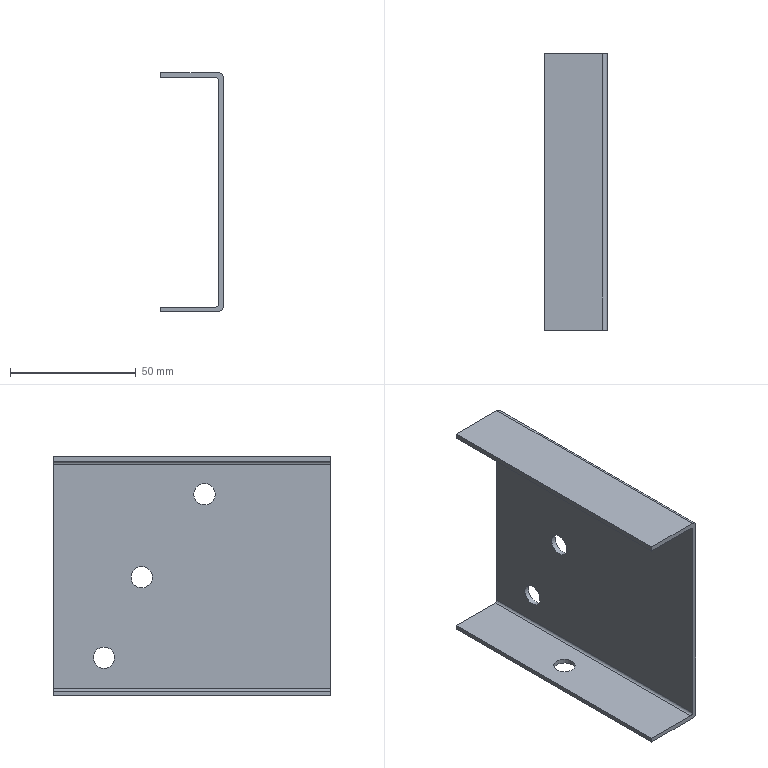Part | STEP file | PN_0066 | 1 solid | 18 faces | box 25 x 110 x 95 mm | volume 29808 mm3 | plane 10 | cylinder 8 | commonest cylinder face diameters 8.5 x4 2 x2 4 x2
STEP:
#1=CARTESIAN_POINT('',(0.,0.,0.));
#2=DIRECTION('',(0.,0.,1.));
#3=DIRECTION('',(1.,0.,0.));
#4=AXIS2_PLACEMENT_3D('',#1,#2,#3);
#5=CARTESIAN_POINT('',(-41.283,0.,45.169));
#6=VERTEX_POINT('',#5);
#7=CARTESIAN_POINT('',(-41.283,0.,43.169));
#8=VERTEX_POINT('',#7);
#9=CARTESIAN_POINT('',(-41.283,0.,43.169));
#10=DIRECTION('',(0.,0.,-1.));
#11=VECTOR('',#10,1.);
#12=LINE('',#9,#11);
#13=CARTESIAN_POINT('',(-41.283,110.,43.169));
#14=DIRECTION('',(1.,0.,0.));
#15=DIRECTION('',(0.,0.,1.));
#16=AXIS2_PLACEMENT_3D('',#13,#14,#15);
#17=PLANE('',#16);
#18=CARTESIAN_POINT('',(0.,110.));
#19=DIRECTION('',(-1.,0.));
#20=VECTOR('',#19,1.);
#21=LINE('',#18,#20);
#22=(GEOMETRIC_REPRESENTATION_CONTEXT(2)PARAMETRIC_REPRESENTATION_CONTEXT()REPRESENTATION_CONTEXT('',''));
#23=DEFINITIONAL_REPRESENTATION('',(#21),#22);
#24=PCURVE('',#17,#23);
#25=CARTESIAN_POINT('',(-18.283,0.,43.169));
#26=DIRECTION('',(0.,1.,0.));
#27=DIRECTION('',(0.,0.,1.));
#28=AXIS2_PLACEMENT_3D('',#25,#26,#27);
#29=PLANE('',#28);
#30=CARTESIAN_POINT('',(0.,-23.));
#31=DIRECTION('',(-1.,0.));
#32=VECTOR('',#31,1.);
#33=LINE('',#30,#32);
#34=(GEOMETRIC_REPRESENTATION_CONTEXT(2)PARAMETRIC_REPRESENTATION_CONTEXT()REPRESENTATION_CONTEXT('',''));
#35=DEFINITIONAL_REPRESENTATION('',(#33),#34);
#36=PCURVE('',#29,#35);
#37=SURFACE_CURVE('',#12,(#24,#36),.PCURVE_S1.);
#38=EDGE_CURVE('',#6,#8,#37,.T.);
#39=ORIENTED_EDGE('',*,*,#38,.F.);
#40=CARTESIAN_POINT('',(-41.283,110.,45.169));
#41=VERTEX_POINT('',#40);
#42=CARTESIAN_POINT('',(-41.283,110.,45.169));
#43=DIRECTION('',(0.,-1.,0.));
#44=VECTOR('',#43,1.);
#45=LINE('',#42,#44);
#46=CARTESIAN_POINT('',(2.,0.));
#47=DIRECTION('',(0.,1.));
#48=VECTOR('',#47,1.);
#49=LINE('',#46,#48);
#50=(GEOMETRIC_REPRESENTATION_CONTEXT(2)PARAMETRIC_REPRESENTATION_CONTEXT()REPRESENTATION_CONTEXT('',''));
#51=DEFINITIONAL_REPRESENTATION('',(#49),#50);
#52=PCURVE('',#17,#51);
#53=CARTESIAN_POINT('',(-18.283,110.,45.169));
#54=DIRECTION('',(0.,0.,-1.));
#55=DIRECTION('',(1.,0.,0.));
#56=AXIS2_PLACEMENT_3D('',#53,#54,#55);
#57=PLANE('',#56);
#58=CARTESIAN_POINT('',(-23.,0.));
#59=DIRECTION('',(0.,1.));
#60=VECTOR('',#59,1.);
#61=LINE('',#58,#60);
#62=(GEOMETRIC_REPRESENTATION_CONTEXT(2)PARAMETRIC_REPRESENTATION_CONTEXT()REPRESENTATION_CONTEXT('',''));
#63=DEFINITIONAL_REPRESENTATION('',(#61),#62);
#64=PCURVE('',#57,#63);
#65=SURFACE_CURVE('',#45,(#52,#64),.PCURVE_S1.);
#66=EDGE_CURVE('',#41,#6,#65,.T.);
#67=ORIENTED_EDGE('',*,*,#66,.F.);
#68=CARTESIAN_POINT('',(-41.283,110.,43.169));
#69=VERTEX_POINT('',#68);
#70=CARTESIAN_POINT('',(-41.283,110.,43.169));
#71=DIRECTION('',(0.,0.,-1.));
#72=VECTOR('',#71,1.);
#73=LINE('',#70,#72);
#74=CARTESIAN_POINT('',(0.,0.));
#75=DIRECTION('',(-1.,0.));
#76=VECTOR('',#75,1.);
#77=LINE('',#74,#76);
#78=(GEOMETRIC_REPRESENTATION_CONTEXT(2)PARAMETRIC_REPRESENTATION_CONTEXT()REPRESENTATION_CONTEXT('',''));
#79=DEFINITIONAL_REPRESENTATION('',(#77),#78);
#80=PCURVE('',#17,#79);
#81=CARTESIAN_POINT('',(-18.283,110.,43.169));
#82=DIRECTION('',(0.,1.,0.));
#83=DIRECTION('',(0.,0.,1.));
#84=AXIS2_PLACEMENT_3D('',#81,#82,#83);
#85=PLANE('',#84);
#86=CARTESIAN_POINT('',(0.,-23.));
#87=DIRECTION('',(-1.,0.));
#88=VECTOR('',#87,1.);
#89=LINE('',#86,#88);
#90=(GEOMETRIC_REPRESENTATION_CONTEXT(2)PARAMETRIC_REPRESENTATION_CONTEXT()REPRESENTATION_CONTEXT('',''));
#91=DEFINITIONAL_REPRESENTATION('',(#89),#90);
#92=PCURVE('',#85,#91);
#93=SURFACE_CURVE('',#73,(#80,#92),.PCURVE_S1.);
#94=EDGE_CURVE('',#41,#69,#93,.T.);
#95=ORIENTED_EDGE('',*,*,#94,.T.);
#96=CARTESIAN_POINT('',(-41.283,110.,43.169));
#97=DIRECTION('',(0.,-1.,0.));
#98=VECTOR('',#97,1.);
#99=LINE('',#96,#98);
#100=CARTESIAN_POINT('',(0.,0.));
#101=DIRECTION('',(0.,1.));
#102=VECTOR('',#101,1.);
#103=LINE('',#100,#102);
#104=(GEOMETRIC_REPRESENTATION_CONTEXT(2)PARAMETRIC_REPRESENTATION_CONTEXT()REPRESENTATION_CONTEXT('',''));
#105=DEFINITIONAL_REPRESENTATION('',(#103),#104);
#106=PCURVE('',#17,#105);
#107=CARTESIAN_POINT('',(-19.283,110.,43.169));
#108=DIRECTION('',(0.,0.,1.));
#109=DIRECTION('',(-1.,0.,0.));
#110=AXIS2_PLACEMENT_3D('',#107,#108,#109);
#111=PLANE('',#110);
#112=CARTESIAN_POINT('',(22.,0.));
#113=DIRECTION('',(0.,1.));
#114=VECTOR('',#113,1.);
#115=LINE('',#112,#114);
#116=(GEOMETRIC_REPRESENTATION_CONTEXT(2)PARAMETRIC_REPRESENTATION_CONTEXT()REPRESENTATION_CONTEXT('',''));
#117=DEFINITIONAL_REPRESENTATION('',(#115),#116);
#118=PCURVE('',#111,#117);
#119=SURFACE_CURVE('',#99,(#106,#118),.PCURVE_S1.);
#120=EDGE_CURVE('',#69,#8,#119,.T.);
#121=ORIENTED_EDGE('',*,*,#120,.T.);
#122=EDGE_LOOP('',(#39,#67,#95,#121));
#123=FACE_BOUND('',#122,.T.);
#124=ADVANCED_FACE('',(#123),#17,.F.);
#125=CARTESIAN_POINT('',(-19.283,0.,43.169));
#126=VERTEX_POINT('',#125);
#127=CARTESIAN_POINT('',(-19.283,0.,43.169));
#128=DIRECTION('',(1.,0.,0.));
#129=VECTOR('',#128,1.);
#130=LINE('',#127,#129);
#131=CARTESIAN_POINT('',(0.,110.));
#132=DIRECTION('',(-1.,0.));
#133=VECTOR('',#132,1.);
#134=LINE('',#131,#133);
#135=(GEOMETRIC_REPRESENTATION_CONTEXT(2)PARAMETRIC_REPRESENTATION_CONTEXT()REPRESENTATION_CONTEXT('',''));
#136=DEFINITIONAL_REPRESENTATION('',(#134),#135);
#137=PCURVE('',#111,#136);
#138=CARTESIAN_POINT('',(0.,-1.));
#139=DIRECTION('',(0.,1.));
#140=VECTOR('',#139,1.);
#141=LINE('',#138,#140);
#142=(GEOMETRIC_REPRESENTATION_CONTEXT(2)PARAMETRIC_REPRESENTATION_CONTEXT()REPRESENTATION_CONTEXT('',''));
#143=DEFINITIONAL_REPRESENTATION('',(#141),#142);
#144=PCURVE('',#29,#143);
#145=SURFACE_CURVE('',#130,(#137,#144),.PCURVE_S1.);
#146=EDGE_CURVE('',#8,#126,#145,.T.);
#147=ORIENTED_EDGE('',*,*,#146,.F.);
#148=ORIENTED_EDGE('',*,*,#120,.F.);
#149=CARTESIAN_POINT('',(-19.283,110.,43.169));
#150=VERTEX_POINT('',#149);
#151=CARTESIAN_POINT('',(-19.283,110.,43.169));
#152=DIRECTION('',(1.,0.,0.));
#153=VECTOR('',#152,1.);
#154=LINE('',#151,#153);
#155=CARTESIAN_POINT('',(0.,0.));
#156=DIRECTION('',(-1.,0.));
#157=VECTOR('',#156,1.);
#158=LINE('',#155,#157);
#159=(GEOMETRIC_REPRESENTATION_CONTEXT(2)PARAMETRIC_REPRESENTATION_CONTEXT()REPRESENTATION_CONTEXT('',''));
#160=DEFINITIONAL_REPRESENTATION('',(#158),#159);
#161=PCURVE('',#111,#160);
#162=CARTESIAN_POINT('',(0.,-1.));
#163=DIRECTION('',(0.,1.));
#164=VECTOR('',#163,1.);
#165=LINE('',#162,#164);
#166=(GEOMETRIC_REPRESENTATION_CONTEXT(2)PARAMETRIC_REPRESENTATION_CONTEXT()REPRESENTATION_CONTEXT('',''));
#167=DEFINITIONAL_REPRESENTATION('',(#165),#166);
#168=PCURVE('',#85,#167);
#169=SURFACE_CURVE('',#154,(#161,#168),.PCURVE_S1.);
#170=EDGE_CURVE('',#69,#150,#169,.T.);
#171=ORIENTED_EDGE('',*,*,#170,.T.);
#172=CARTESIAN_POINT('',(-19.283,110.,43.169));
#173=DIRECTION('',(0.,-1.,0.));
#174=VECTOR('',#173,1.);
#175=LINE('',#172,#174);
#176=CARTESIAN_POINT('',(0.,0.));
#177=DIRECTION('',(0.,1.));
#178=VECTOR('',#177,1.);
#179=LINE('',#176,#178);
#180=(GEOMETRIC_REPRESENTATION_CONTEXT(2)PARAMETRIC_REPRESENTATION_CONTEXT()REPRESENTATION_CONTEXT('',''));
#181=DEFINITIONAL_REPRESENTATION('',(#179),#180);
#182=PCURVE('',#111,#181);
#183=CARTESIAN_POINT('',(-19.283,110.,42.169));
#184=DIRECTION('',(0.,-1.,0.));
#185=DIRECTION('',(0.,0.,-1.));
#186=AXIS2_PLACEMENT_3D('',#183,#184,#185);
#187=CYLINDRICAL_SURFACE('',#186,1.);
#188=CARTESIAN_POINT('',(3.142,0.));
#189=DIRECTION('',(0.,1.));
#190=VECTOR('',#189,1.);
#191=LINE('',#188,#190);
#192=(GEOMETRIC_REPRESENTATION_CONTEXT(2)PARAMETRIC_REPRESENTATION_CONTEXT()REPRESENTATION_CONTEXT('',''));
#193=DEFINITIONAL_REPRESENTATION('',(#191),#192);
#194=PCURVE('',#187,#193);
#195=SURFACE_CURVE('',#175,(#182,#194),.PCURVE_S1.);
#196=EDGE_CURVE('',#150,#126,#195,.T.);
#197=ORIENTED_EDGE('',*,*,#196,.T.);
#198=EDGE_LOOP('',(#147,#148,#171,#197));
#199=FACE_BOUND('',#198,.T.);
#200=ADVANCED_FACE('',(#199),#111,.F.);
#201=CARTESIAN_POINT('',(-18.283,110.,42.169));
#202=VERTEX_POINT('',#201);
#203=CARTESIAN_POINT('',(-18.283,0.,42.169));
#204=VERTEX_POINT('',#203);
#205=CARTESIAN_POINT('',(-18.283,110.,42.169));
#206=DIRECTION('',(0.,-1.,0.));
#207=VECTOR('',#206,1.);
#208=LINE('',#205,#207);
#209=CARTESIAN_POINT('',(1.571,0.));
#210=DIRECTION('',(0.,1.));
#211=VECTOR('',#210,1.);
#212=LINE('',#209,#211);
#213=(GEOMETRIC_REPRESENTATION_CONTEXT(2)PARAMETRIC_REPRESENTATION_CONTEXT()REPRESENTATION_CONTEXT('',''));
#214=DEFINITIONAL_REPRESENTATION('',(#212),#213);
#215=PCURVE('',#187,#214);
#216=CARTESIAN_POINT('',(-18.283,110.,-47.08));
#217=DIRECTION('',(1.,0.,0.));
#218=DIRECTION('',(0.,0.,1.));
#219=AXIS2_PLACEMENT_3D('',#216,#217,#218);
#220=PLANE('',#219);
#221=CARTESIAN_POINT('',(89.249,0.));
#222=DIRECTION('',(0.,1.));
#223=VECTOR('',#222,1.);
#224=LINE('',#221,#223);
#225=(GEOMETRIC_REPRESENTATION_CONTEXT(2)PARAMETRIC_REPRESENTATION_CONTEXT()REPRESENTATION_CONTEXT('',''));
#226=DEFINITIONAL_REPRESENTATION('',(#224),#225);
#227=PCURVE('',#220,#226);
#228=SURFACE_CURVE('',#208,(#215,#227),.PCURVE_S1.);
#229=EDGE_CURVE('',#202,#204,#228,.T.);
#230=ORIENTED_EDGE('',*,*,#229,.F.);
#231=CARTESIAN_POINT('',(-19.283,110.,42.169));
#232=DIRECTION('',(0.,1.,0.));
#233=DIRECTION('',(0.,0.,1.));
#234=AXIS2_PLACEMENT_3D('',#231,#232,#233);
#235=CIRCLE('',#234,1.);
#236=CARTESIAN_POINT('',(3.142,0.));
#237=DIRECTION('',(-1.,0.));
#238=VECTOR('',#237,1.);
#239=LINE('',#236,#238);
#240=(GEOMETRIC_REPRESENTATION_CONTEXT(2)PARAMETRIC_REPRESENTATION_CONTEXT()REPRESENTATION_CONTEXT('',''));
#241=DEFINITIONAL_REPRESENTATION('',(#239),#240);
#242=PCURVE('',#187,#241);
#243=CARTESIAN_POINT('',(-1.,-1.));
#244=DIRECTION('',(1.,0.));
#245=AXIS2_PLACEMENT_2D('',#243,#244);
#246=CIRCLE('',#245,1.);
#247=(GEOMETRIC_REPRESENTATION_CONTEXT(2)PARAMETRIC_REPRESENTATION_CONTEXT()REPRESENTATION_CONTEXT('',''));
#248=DEFINITIONAL_REPRESENTATION('',(#246),#247);
#249=PCURVE('',#85,#248);
#250=SURFACE_CURVE('',#235,(#242,#249),.PCURVE_S1.);
#251=EDGE_CURVE('',#150,#202,#250,.T.);
#252=ORIENTED_EDGE('',*,*,#251,.F.);
#253=ORIENTED_EDGE('',*,*,#196,.T.);
#254=CARTESIAN_POINT('',(-19.283,0.,42.169));
#255=DIRECTION('',(0.,1.,0.));
#256=DIRECTION('',(0.,0.,1.));
#257=AXIS2_PLACEMENT_3D('',#254,#255,#256);
#258=CIRCLE('',#257,1.);
#259=CARTESIAN_POINT('',(3.142,110.));
#260=DIRECTION('',(-1.,0.));
#261=VECTOR('',#260,1.);
#262=LINE('',#259,#261);
#263=(GEOMETRIC_REPRESENTATION_CONTEXT(2)PARAMETRIC_REPRESENTATION_CONTEXT()REPRESENTATION_CONTEXT('',''));
#264=DEFINITIONAL_REPRESENTATION('',(#262),#263);
#265=PCURVE('',#187,#264);
#266=CARTESIAN_POINT('',(-1.,-1.));
#267=DIRECTION('',(1.,0.));
#268=AXIS2_PLACEMENT_2D('',#266,#267);
#269=CIRCLE('',#268,1.);
#270=(GEOMETRIC_REPRESENTATION_CONTEXT(2)PARAMETRIC_REPRESENTATION_CONTEXT()REPRESENTATION_CONTEXT('',''));
#271=DEFINITIONAL_REPRESENTATION('',(#269),#270);
#272=PCURVE('',#29,#271);
#273=SURFACE_CURVE('',#258,(#265,#272),.PCURVE_S1.);
#274=EDGE_CURVE('',#126,#204,#273,.T.);
#275=ORIENTED_EDGE('',*,*,#274,.T.);
#276=EDGE_LOOP('',(#230,#252,#253,#275));
#277=FACE_BOUND('',#276,.F.);
#278=ADVANCED_FACE('',(#277),#187,.F.);
#279=CARTESIAN_POINT('',(-18.283,75.,-7.081));
#280=VERTEX_POINT('',#279);
#281=CARTESIAN_POINT('',(-18.283,75.,-2.831));
#282=DIRECTION('',(1.,0.,0.));
#283=DIRECTION('',(0.,0.,-1.));
#284=AXIS2_PLACEMENT_3D('',#281,#282,#283);
#285=CIRCLE('',#284,4.25);
#286=CARTESIAN_POINT('',(44.249,35.));
#287=DIRECTION('',(-1.,0.));
#288=AXIS2_PLACEMENT_2D('',#286,#287);
#289=CIRCLE('',#288,4.25);
#290=(GEOMETRIC_REPRESENTATION_CONTEXT(2)PARAMETRIC_REPRESENTATION_CONTEXT()REPRESENTATION_CONTEXT('',''));
#291=DEFINITIONAL_REPRESENTATION('',(#289),#290);
#292=PCURVE('',#220,#291);
#293=CARTESIAN_POINT('',(-8.283,75.,-2.831));
#294=DIRECTION('',(-1.,0.,0.));
#295=DIRECTION('',(0.,0.,-1.));
#296=AXIS2_PLACEMENT_3D('',#293,#294,#295);
#297=CYLINDRICAL_SURFACE('',#296,4.25);
#298=CARTESIAN_POINT('',(6.283,10.));
#299=DIRECTION('',(-1.,0.));
#300=VECTOR('',#299,1.);
#301=LINE('',#298,#300);
#302=(GEOMETRIC_REPRESENTATION_CONTEXT(2)PARAMETRIC_REPRESENTATION_CONTEXT()REPRESENTATION_CONTEXT('',''));
#303=DEFINITIONAL_REPRESENTATION('',(#301),#302);
#304=PCURVE('',#297,#303);
#305=SURFACE_CURVE('',#285,(#292,#304),.PCURVE_S1.);
#306=EDGE_CURVE('',#280,#280,#305,.T.);
#307=ORIENTED_EDGE('',*,*,#306,.T.);
#308=EDGE_LOOP('',(#307));
#309=FACE_BOUND('',#308,.T.);
#310=CARTESIAN_POINT('',(-18.283,50.,25.919));
#311=VERTEX_POINT('',#310);
#312=CARTESIAN_POINT('',(-18.283,50.,30.169));
#313=DIRECTION('',(1.,0.,0.));
#314=DIRECTION('',(0.,0.,-1.));
#315=AXIS2_PLACEMENT_3D('',#312,#313,#314);
#316=CIRCLE('',#315,4.25);
#317=CARTESIAN_POINT('',(77.249,60.));
#318=DIRECTION('',(-1.,0.));
#319=AXIS2_PLACEMENT_2D('',#317,#318);
#320=CIRCLE('',#319,4.25);
#321=(GEOMETRIC_REPRESENTATION_CONTEXT(2)PARAMETRIC_REPRESENTATION_CONTEXT()REPRESENTATION_CONTEXT('',''));
#322=DEFINITIONAL_REPRESENTATION('',(#320),#321);
#323=PCURVE('',#220,#322);
#324=CARTESIAN_POINT('',(-8.283,50.,30.169));
#325=DIRECTION('',(-1.,0.,0.));
#326=DIRECTION('',(0.,0.,-1.));
#327=AXIS2_PLACEMENT_3D('',#324,#325,#326);
#328=CYLINDRICAL_SURFACE('',#327,4.25);
#329=CARTESIAN_POINT('',(6.283,10.));
#330=DIRECTION('',(-1.,0.));
#331=VECTOR('',#330,1.);
#332=LINE('',#329,#331);
#333=(GEOMETRIC_REPRESENTATION_CONTEXT(2)PARAMETRIC_REPRESENTATION_CONTEXT()REPRESENTATION_CONTEXT('',''));
#334=DEFINITIONAL_REPRESENTATION('',(#332),#333);
#335=PCURVE('',#328,#334);
#336=SURFACE_CURVE('',#316,(#323,#335),.PCURVE_S1.);
#337=EDGE_CURVE('',#311,#311,#336,.T.);
#338=ORIENTED_EDGE('',*,*,#337,.T.);
#339=EDGE_LOOP('',(#338));
#340=FACE_BOUND('',#339,.T.);
#341=CARTESIAN_POINT('',(-18.283,90.,-39.081));
#342=VERTEX_POINT('',#341);
#343=CARTESIAN_POINT('',(-18.283,90.,-34.831));
#344=DIRECTION('',(1.,0.,0.));
#345=DIRECTION('',(0.,0.,-1.));
#346=AXIS2_PLACEMENT_3D('',#343,#344,#345);
#347=CIRCLE('',#346,4.25);
#348=CARTESIAN_POINT('',(12.249,20.));
#349=DIRECTION('',(-1.,0.));
#350=AXIS2_PLACEMENT_2D('',#348,#349);
#351=CIRCLE('',#350,4.25);
#352=(GEOMETRIC_REPRESENTATION_CONTEXT(2)PARAMETRIC_REPRESENTATION_CONTEXT()REPRESENTATION_CONTEXT('',''));
#353=DEFINITIONAL_REPRESENTATION('',(#351),#352);
#354=PCURVE('',#220,#353);
#355=CARTESIAN_POINT('',(-8.283,90.,-34.831));
#356=DIRECTION('',(-1.,0.,0.));
#357=DIRECTION('',(0.,0.,-1.));
#358=AXIS2_PLACEMENT_3D('',#355,#356,#357);
#359=CYLINDRICAL_SURFACE('',#358,4.25);
#360=CARTESIAN_POINT('',(6.283,10.));
#361=DIRECTION('',(-1.,0.));
#362=VECTOR('',#361,1.);
#363=LINE('',#360,#362);
#364=(GEOMETRIC_REPRESENTATION_CONTEXT(2)PARAMETRIC_REPRESENTATION_CONTEXT()REPRESENTATION_CONTEXT('',''));
#365=DEFINITIONAL_REPRESENTATION('',(#363),#364);
#366=PCURVE('',#359,#365);
#367=SURFACE_CURVE('',#347,(#354,#366),.PCURVE_S1.);
#368=EDGE_CURVE('',#342,#342,#367,.T.);
#369=ORIENTED_EDGE('',*,*,#368,.T.);
#370=EDGE_LOOP('',(#369));
#371=FACE_BOUND('',#370,.T.);
#372=CARTESIAN_POINT('',(-18.283,0.,-47.08));
#373=VERTEX_POINT('',#372);
#374=CARTESIAN_POINT('',(-18.283,0.,-47.08));
#375=DIRECTION('',(0.,0.,-1.));
#376=VECTOR('',#375,1.);
#377=LINE('',#374,#376);
#378=CARTESIAN_POINT('',(0.,110.));
#379=DIRECTION('',(-1.,0.));
#380=VECTOR('',#379,1.);
#381=LINE('',#378,#380);
#382=(GEOMETRIC_REPRESENTATION_CONTEXT(2)PARAMETRIC_REPRESENTATION_CONTEXT()REPRESENTATION_CONTEXT('',''));
#383=DEFINITIONAL_REPRESENTATION('',(#381),#382);
#384=PCURVE('',#220,#383);
#385=CARTESIAN_POINT('',(-90.249,0.));
#386=DIRECTION('',(-1.,0.));
#387=VECTOR('',#386,1.);
#388=LINE('',#385,#387);
#389=(GEOMETRIC_REPRESENTATION_CONTEXT(2)PARAMETRIC_REPRESENTATION_CONTEXT()REPRESENTATION_CONTEXT('',''));
#390=DEFINITIONAL_REPRESENTATION('',(#388),#389);
#391=PCURVE('',#29,#390);
#392=SURFACE_CURVE('',#377,(#384,#391),.PCURVE_S1.);
#393=EDGE_CURVE('',#204,#373,#392,.T.);
#394=ORIENTED_EDGE('',*,*,#393,.F.);
#395=ORIENTED_EDGE('',*,*,#229,.F.);
#396=CARTESIAN_POINT('',(-18.283,110.,-47.08));
#397=VERTEX_POINT('',#396);
#398=CARTESIAN_POINT('',(-18.283,110.,-47.08));
#399=DIRECTION('',(0.,0.,-1.));
#400=VECTOR('',#399,1.);
#401=LINE('',#398,#400);
#402=CARTESIAN_POINT('',(0.,0.));
#403=DIRECTION('',(-1.,0.));
#404=VECTOR('',#403,1.);
#405=LINE('',#402,#404);
#406=(GEOMETRIC_REPRESENTATION_CONTEXT(2)PARAMETRIC_REPRESENTATION_CONTEXT()REPRESENTATION_CONTEXT('',''));
#407=DEFINITIONAL_REPRESENTATION('',(#405),#406);
#408=PCURVE('',#220,#407);
#409=CARTESIAN_POINT('',(-90.249,0.));
#410=DIRECTION('',(-1.,0.));
#411=VECTOR('',#410,1.);
#412=LINE('',#409,#411);
#413=(GEOMETRIC_REPRESENTATION_CONTEXT(2)PARAMETRIC_REPRESENTATION_CONTEXT()REPRESENTATION_CONTEXT('',''));
#414=DEFINITIONAL_REPRESENTATION('',(#412),#413);
#415=PCURVE('',#85,#414);
#416=SURFACE_CURVE('',#401,(#408,#415),.PCURVE_S1.);
#417=EDGE_CURVE('',#202,#397,#416,.T.);
#418=ORIENTED_EDGE('',*,*,#417,.T.);
#419=CARTESIAN_POINT('',(-18.283,110.,-47.08));
#420=DIRECTION('',(0.,-1.,0.));
#421=VECTOR('',#420,1.);
#422=LINE('',#419,#421);
#423=CARTESIAN_POINT('',(0.,0.));
#424=DIRECTION('',(0.,1.));
#425=VECTOR('',#424,1.);
#426=LINE('',#423,#425);
#427=(GEOMETRIC_REPRESENTATION_CONTEXT(2)PARAMETRIC_REPRESENTATION_CONTEXT()REPRESENTATION_CONTEXT('',''));
#428=DEFINITIONAL_REPRESENTATION('',(#426),#427);
#429=PCURVE('',#220,#428);
#430=CARTESIAN_POINT('',(-19.283,110.,-47.08));
#431=DIRECTION('',(0.,-1.,0.));
#432=DIRECTION('',(0.,0.,-1.));
#433=AXIS2_PLACEMENT_3D('',#430,#431,#432);
#434=CYLINDRICAL_SURFACE('',#433,1.);
#435=CARTESIAN_POINT('',(1.571,0.));
#436=DIRECTION('',(0.,1.));
#437=VECTOR('',#436,1.);
#438=LINE('',#435,#437);
#439=(GEOMETRIC_REPRESENTATION_CONTEXT(2)PARAMETRIC_REPRESENTATION_CONTEXT()REPRESENTATION_CONTEXT('',''));
#440=DEFINITIONAL_REPRESENTATION('',(#438),#439);
#441=PCURVE('',#434,#440);
#442=SURFACE_CURVE('',#422,(#429,#441),.PCURVE_S1.);
#443=EDGE_CURVE('',#397,#373,#442,.T.);
#444=ORIENTED_EDGE('',*,*,#443,.T.);
#445=EDGE_LOOP('',(#394,#395,#418,#444));
#446=FACE_BOUND('',#445,.T.);
#447=ADVANCED_FACE('',(#309,#340,#371,#446),#220,.F.);
#448=CARTESIAN_POINT('',(-19.283,110.,-48.08));
#449=VERTEX_POINT('',#448);
#450=CARTESIAN_POINT('',(-19.283,0.,-48.08));
#451=VERTEX_POINT('',#450);
#452=CARTESIAN_POINT('',(-19.283,110.,-48.08));
#453=DIRECTION('',(0.,-1.,0.));
#454=VECTOR('',#453,1.);
#455=LINE('',#452,#454);
#456=CARTESIAN_POINT('',(0.,0.));
#457=DIRECTION('',(0.,1.));
#458=VECTOR('',#457,1.);
#459=LINE('',#456,#458);
#460=(GEOMETRIC_REPRESENTATION_CONTEXT(2)PARAMETRIC_REPRESENTATION_CONTEXT()REPRESENTATION_CONTEXT('',''));
#461=DEFINITIONAL_REPRESENTATION('',(#459),#460);
#462=PCURVE('',#434,#461);
#463=CARTESIAN_POINT('',(-19.283,110.,-48.08));
#464=DIRECTION('',(0.,0.,-1.));
#465=DIRECTION('',(1.,0.,0.));
#466=AXIS2_PLACEMENT_3D('',#463,#464,#465);
#467=PLANE('',#466);
#468=CARTESIAN_POINT('',(0.,0.));
#469=DIRECTION('',(0.,1.));
#470=VECTOR('',#469,1.);
#471=LINE('',#468,#470);
#472=(GEOMETRIC_REPRESENTATION_CONTEXT(2)PARAMETRIC_REPRESENTATION_CONTEXT()REPRESENTATION_CONTEXT('',''));
#473=DEFINITIONAL_REPRESENTATION('',(#471),#472);
#474=PCURVE('',#467,#473);
#475=SURFACE_CURVE('',#455,(#462,#474),.PCURVE_S1.);
#476=EDGE_CURVE('',#449,#451,#475,.T.);
#477=ORIENTED_EDGE('',*,*,#476,.F.);
#478=CARTESIAN_POINT('',(-19.283,110.,-47.08));
#479=DIRECTION('',(0.,1.,0.));
#480=DIRECTION('',(0.,0.,-1.));
#481=AXIS2_PLACEMENT_3D('',#478,#479,#480);
#482=CIRCLE('',#481,1.);
#483=CARTESIAN_POINT('',(6.283,0.));
#484=DIRECTION('',(-1.,0.));
#485=VECTOR('',#484,1.);
#486=LINE('',#483,#485);
#487=(GEOMETRIC_REPRESENTATION_CONTEXT(2)PARAMETRIC_REPRESENTATION_CONTEXT()REPRESENTATION_CONTEXT('',''));
#488=DEFINITIONAL_REPRESENTATION('',(#486),#487);
#489=PCURVE('',#434,#488);
#490=CARTESIAN_POINT('',(-90.249,-1.));
#491=DIRECTION('',(-1.,0.));
#492=AXIS2_PLACEMENT_2D('',#490,#491);
#493=CIRCLE('',#492,1.);
#494=(GEOMETRIC_REPRESENTATION_CONTEXT(2)PARAMETRIC_REPRESENTATION_CONTEXT()REPRESENTATION_CONTEXT('',''));
#495=DEFINITIONAL_REPRESENTATION('',(#493),#494);
#496=PCURVE('',#85,#495);
#497=SURFACE_CURVE('',#482,(#489,#496),.PCURVE_S1.);
#498=EDGE_CURVE('',#397,#449,#497,.T.);
#499=ORIENTED_EDGE('',*,*,#498,.F.);
#500=ORIENTED_EDGE('',*,*,#443,.T.);
#501=CARTESIAN_POINT('',(-19.283,0.,-47.08));
#502=DIRECTION('',(0.,1.,0.));
#503=DIRECTION('',(0.,0.,-1.));
#504=AXIS2_PLACEMENT_3D('',#501,#502,#503);
#505=CIRCLE('',#504,1.);
#506=CARTESIAN_POINT('',(6.283,110.));
#507=DIRECTION('',(-1.,0.));
#508=VECTOR('',#507,1.);
#509=LINE('',#506,#508);
#510=(GEOMETRIC_REPRESENTATION_CONTEXT(2)PARAMETRIC_REPRESENTATION_CONTEXT()REPRESENTATION_CONTEXT('',''));
#511=DEFINITIONAL_REPRESENTATION('',(#509),#510);
#512=PCURVE('',#434,#511);
#513=CARTESIAN_POINT('',(-90.249,-1.));
#514=DIRECTION('',(-1.,0.));
#515=AXIS2_PLACEMENT_2D('',#513,#514);
#516=CIRCLE('',#515,1.);
#517=(GEOMETRIC_REPRESENTATION_CONTEXT(2)PARAMETRIC_REPRESENTATION_CONTEXT()REPRESENTATION_CONTEXT('',''));
#518=DEFINITIONAL_REPRESENTATION('',(#516),#517);
#519=PCURVE('',#29,#518);
#520=SURFACE_CURVE('',#505,(#512,#519),.PCURVE_S1.);
#521=EDGE_CURVE('',#373,#451,#520,.T.);
#522=ORIENTED_EDGE('',*,*,#521,.T.);
#523=EDGE_LOOP('',(#477,#499,#500,#522));
#524=FACE_BOUND('',#523,.F.);
#525=ADVANCED_FACE('',(#524),#434,.F.);
#526=CARTESIAN_POINT('',(-26.033,60.,-48.08));
#527=VERTEX_POINT('',#526);
#528=CARTESIAN_POINT('',(-34.533,60.,-48.08));
#529=VERTEX_POINT('',#528);
#530=CARTESIAN_POINT('',(-30.283,60.,-48.08));
#531=DIRECTION('',(0.,0.,1.));
#532=DIRECTION('',(1.,0.,0.));
#533=AXIS2_PLACEMENT_3D('',#530,#531,#532);
#534=CIRCLE('',#533,4.25);
#535=CARTESIAN_POINT('',(-6.75,50.));
#536=CARTESIAN_POINT('',(-6.75,42.639));
#537=CARTESIAN_POINT('',(-13.125,46.319));
#538=CARTESIAN_POINT('',(-19.5,50.));
#539=CARTESIAN_POINT('',(-13.125,53.681));
#540=CARTESIAN_POINT('',(-6.75,57.361));
#541=CARTESIAN_POINT('',(-6.75,50.));
#542=(BOUNDED_CURVE()B_SPLINE_CURVE(2,(#535,#536,#537,#538,#539,#540,#541),.UNSPECIFIED.,.T.,.F.)B_SPLINE_CURVE_WITH_KNOTS((1,2,2,2,2,1),(-2.094,0.,2.094,4.189,6.283,8.378),.UNSPECIFIED.)CURVE()GEOMETRIC_REPRESENTATION_ITEM()RATIONAL_B_SPLINE_CURVE((1.,0.5,1.,0.5,1.,0.5,1.))REPRESENTATION_ITEM(''));
#543=(GEOMETRIC_REPRESENTATION_CONTEXT(2)PARAMETRIC_REPRESENTATION_CONTEXT()REPRESENTATION_CONTEXT('',''));
#544=DEFINITIONAL_REPRESENTATION('',(#542),#543);
#545=PCURVE('',#467,#544);
#546=CARTESIAN_POINT('',(-30.283,60.,-84.831));
#547=DIRECTION('',(0.,0.,1.));
#548=DIRECTION('',(-1.,0.,0.));
#549=AXIS2_PLACEMENT_3D('',#546,#547,#548);
#550=CYLINDRICAL_SURFACE('',#549,4.25);
#551=CARTESIAN_POINT('',(3.142,36.751));
#552=DIRECTION('',(1.,0.));
#553=VECTOR('',#552,1.);
#554=LINE('',#551,#553);
#555=(GEOMETRIC_REPRESENTATION_CONTEXT(2)PARAMETRIC_REPRESENTATION_CONTEXT()REPRESENTATION_CONTEXT('',''));
#556=DEFINITIONAL_REPRESENTATION('',(#554),#555);
#557=PCURVE('',#550,#556);
#558=SURFACE_CURVE('',#534,(#545,#557),.PCURVE_S1.);
#559=EDGE_CURVE('',#527,#529,#558,.T.);
#560=ORIENTED_EDGE('',*,*,#559,.F.);
#561=CARTESIAN_POINT('',(-30.283,60.,-48.08));
#562=DIRECTION('',(0.,0.,1.));
#563=DIRECTION('',(1.,0.,0.));
#564=AXIS2_PLACEMENT_3D('',#561,#562,#563);
#565=CIRCLE('',#564,4.25);
#566=CARTESIAN_POINT('',(-6.75,50.));
#567=CARTESIAN_POINT('',(-6.75,42.639));
#568=CARTESIAN_POINT('',(-13.125,46.319));
#569=CARTESIAN_POINT('',(-19.5,50.));
#570=CARTESIAN_POINT('',(-13.125,53.681));
#571=CARTESIAN_POINT('',(-6.75,57.361));
#572=CARTESIAN_POINT('',(-6.75,50.));
#573=(BOUNDED_CURVE()B_SPLINE_CURVE(2,(#566,#567,#568,#569,#570,#571,#572),.UNSPECIFIED.,.T.,.F.)B_SPLINE_CURVE_WITH_KNOTS((1,2,2,2,2,1),(-2.094,0.,2.094,4.189,6.283,8.378),.UNSPECIFIED.)CURVE()GEOMETRIC_REPRESENTATION_ITEM()RATIONAL_B_SPLINE_CURVE((1.,0.5,1.,0.5,1.,0.5,1.))REPRESENTATION_ITEM(''));
#574=(GEOMETRIC_REPRESENTATION_CONTEXT(2)PARAMETRIC_REPRESENTATION_CONTEXT()REPRESENTATION_CONTEXT('',''));
#575=DEFINITIONAL_REPRESENTATION('',(#573),#574);
#576=PCURVE('',#467,#575);
#577=CARTESIAN_POINT('',(-3.142,36.751));
#578=DIRECTION('',(1.,0.));
#579=VECTOR('',#578,1.);
#580=LINE('',#577,#579);
#581=(GEOMETRIC_REPRESENTATION_CONTEXT(2)PARAMETRIC_REPRESENTATION_CONTEXT()REPRESENTATION_CONTEXT('',''));
#582=DEFINITIONAL_REPRESENTATION('',(#580),#581);
#583=PCURVE('',#550,#582);
#584=SURFACE_CURVE('',#565,(#576,#583),.PCURVE_S1.);
#585=EDGE_CURVE('',#529,#527,#584,.T.);
#586=ORIENTED_EDGE('',*,*,#585,.F.);
#587=EDGE_LOOP('',(#560,#586));
#588=FACE_BOUND('',#587,.T.);
#589=CARTESIAN_POINT('',(-41.283,0.,-48.08));
#590=VERTEX_POINT('',#589);
#591=CARTESIAN_POINT('',(-19.283,0.,-48.08));
#592=DIRECTION('',(-1.,0.,0.));
#593=VECTOR('',#592,1.);
#594=LINE('',#591,#593);
#595=CARTESIAN_POINT('',(0.,110.));
#596=DIRECTION('',(-1.,0.));
#597=VECTOR('',#596,1.);
#598=LINE('',#595,#597);
#599=(GEOMETRIC_REPRESENTATION_CONTEXT(2)PARAMETRIC_REPRESENTATION_CONTEXT()REPRESENTATION_CONTEXT('',''));
#600=DEFINITIONAL_REPRESENTATION('',(#598),#599);
#601=PCURVE('',#467,#600);
#602=CARTESIAN_POINT('',(-91.249,-1.));
#603=DIRECTION('',(0.,-1.));
#604=VECTOR('',#603,1.);
#605=LINE('',#602,#604);
#606=(GEOMETRIC_REPRESENTATION_CONTEXT(2)PARAMETRIC_REPRESENTATION_CONTEXT()REPRESENTATION_CONTEXT('',''));
#607=DEFINITIONAL_REPRESENTATION('',(#605),#606);
#608=PCURVE('',#29,#607);
#609=SURFACE_CURVE('',#594,(#601,#608),.PCURVE_S1.);
#610=EDGE_CURVE('',#451,#590,#609,.T.);
#611=ORIENTED_EDGE('',*,*,#610,.F.);
#612=ORIENTED_EDGE('',*,*,#476,.F.);
#613=CARTESIAN_POINT('',(-41.283,110.,-48.08));
#614=VERTEX_POINT('',#613);
#615=CARTESIAN_POINT('',(-19.283,110.,-48.08));
#616=DIRECTION('',(-1.,0.,0.));
#617=VECTOR('',#616,1.);
#618=LINE('',#615,#617);
#619=CARTESIAN_POINT('',(0.,0.));
#620=DIRECTION('',(-1.,0.));
#621=VECTOR('',#620,1.);
#622=LINE('',#619,#621);
#623=(GEOMETRIC_REPRESENTATION_CONTEXT(2)PARAMETRIC_REPRESENTATION_CONTEXT()REPRESENTATION_CONTEXT('',''));
#624=DEFINITIONAL_REPRESENTATION('',(#622),#623);
#625=PCURVE('',#467,#624);
#626=CARTESIAN_POINT('',(-91.249,-1.));
#627=DIRECTION('',(0.,-1.));
#628=VECTOR('',#627,1.);
#629=LINE('',#626,#628);
#630=(GEOMETRIC_REPRESENTATION_CONTEXT(2)PARAMETRIC_REPRESENTATION_CONTEXT()REPRESENTATION_CONTEXT('',''));
#631=DEFINITIONAL_REPRESENTATION('',(#629),#630);
#632=PCURVE('',#85,#631);
#633=SURFACE_CURVE('',#618,(#625,#632),.PCURVE_S1.);
#634=EDGE_CURVE('',#449,#614,#633,.T.);
#635=ORIENTED_EDGE('',*,*,#634,.T.);
#636=CARTESIAN_POINT('',(-41.283,110.,-48.08));
#637=DIRECTION('',(0.,-1.,0.));
#638=VECTOR('',#637,1.);
#639=LINE('',#636,#638);
#640=CARTESIAN_POINT('',(-22.,0.));
#641=DIRECTION('',(0.,1.));
#642=VECTOR('',#641,1.);
#643=LINE('',#640,#642);
#644=(GEOMETRIC_REPRESENTATION_CONTEXT(2)PARAMETRIC_REPRESENTATION_CONTEXT()REPRESENTATION_CONTEXT('',''));
#645=DEFINITIONAL_REPRESENTATION('',(#643),#644);
#646=PCURVE('',#467,#645);
#647=CARTESIAN_POINT('',(-41.283,110.,-48.08));
#648=DIRECTION('',(1.,0.,0.));
#649=DIRECTION('',(0.,0.,1.));
#650=AXIS2_PLACEMENT_3D('',#647,#648,#649);
#651=PLANE('',#650);
#652=CARTESIAN_POINT('',(0.,0.));
#653=DIRECTION('',(0.,1.));
#654=VECTOR('',#653,1.);
#655=LINE('',#652,#654);
#656=(GEOMETRIC_REPRESENTATION_CONTEXT(2)PARAMETRIC_REPRESENTATION_CONTEXT()REPRESENTATION_CONTEXT('',''));
#657=DEFINITIONAL_REPRESENTATION('',(#655),#656);
#658=PCURVE('',#651,#657);
#659=SURFACE_CURVE('',#639,(#646,#658),.PCURVE_S1.);
#660=EDGE_CURVE('',#614,#590,#659,.T.);
#661=ORIENTED_EDGE('',*,*,#660,.T.);
#662=EDGE_LOOP('',(#611,#612,#635,#661));
#663=FACE_BOUND('',#662,.T.);
#664=ADVANCED_FACE('',(#588,#663),#467,.F.);
#665=CARTESIAN_POINT('',(-41.283,0.,-49.831));
#666=VERTEX_POINT('',#665);
#667=CARTESIAN_POINT('',(-41.283,0.,-48.08));
#668=DIRECTION('',(0.,0.,-1.));
#669=VECTOR('',#668,1.);
#670=LINE('',#667,#669);
#671=CARTESIAN_POINT('',(0.,110.));
#672=DIRECTION('',(-1.,0.));
#673=VECTOR('',#672,1.);
#674=LINE('',#671,#673);
#675=(GEOMETRIC_REPRESENTATION_CONTEXT(2)PARAMETRIC_REPRESENTATION_CONTEXT()REPRESENTATION_CONTEXT('',''));
#676=DEFINITIONAL_REPRESENTATION('',(#674),#675);
#677=PCURVE('',#651,#676);
#678=CARTESIAN_POINT('',(-91.249,-23.));
#679=DIRECTION('',(-1.,0.));
#680=VECTOR('',#679,1.);
#681=LINE('',#678,#680);
#682=(GEOMETRIC_REPRESENTATION_CONTEXT(2)PARAMETRIC_REPRESENTATION_CONTEXT()REPRESENTATION_CONTEXT('',''));
#683=DEFINITIONAL_REPRESENTATION('',(#681),#682);
#684=PCURVE('',#29,#683);
#685=SURFACE_CURVE('',#670,(#677,#684),.PCURVE_S1.);
#686=EDGE_CURVE('',#590,#666,#685,.T.);
#687=ORIENTED_EDGE('',*,*,#686,.F.);
#688=ORIENTED_EDGE('',*,*,#660,.F.);
#689=CARTESIAN_POINT('',(-41.283,110.,-49.831));
#690=VERTEX_POINT('',#689);
#691=CARTESIAN_POINT('',(-41.283,110.,-48.08));
#692=DIRECTION('',(0.,0.,-1.));
#693=VECTOR('',#692,1.);
#694=LINE('',#691,#693);
#695=CARTESIAN_POINT('',(0.,0.));
#696=DIRECTION('',(-1.,0.));
#697=VECTOR('',#696,1.);
#698=LINE('',#695,#697);
#699=(GEOMETRIC_REPRESENTATION_CONTEXT(2)PARAMETRIC_REPRESENTATION_CONTEXT()REPRESENTATION_CONTEXT('',''));
#700=DEFINITIONAL_REPRESENTATION('',(#698),#699);
#701=PCURVE('',#651,#700);
#702=CARTESIAN_POINT('',(-91.249,-23.));
#703=DIRECTION('',(-1.,0.));
#704=VECTOR('',#703,1.);
#705=LINE('',#702,#704);
#706=(GEOMETRIC_REPRESENTATION_CONTEXT(2)PARAMETRIC_REPRESENTATION_CONTEXT()REPRESENTATION_CONTEXT('',''));
#707=DEFINITIONAL_REPRESENTATION('',(#705),#706);
#708=PCURVE('',#85,#707);
#709=SURFACE_CURVE('',#694,(#701,#708),.PCURVE_S1.);
#710=EDGE_CURVE('',#614,#690,#709,.T.);
#711=ORIENTED_EDGE('',*,*,#710,.T.);
#712=CARTESIAN_POINT('',(-41.283,110.,-49.831));
#713=DIRECTION('',(0.,-1.,0.));
#714=VECTOR('',#713,1.);
#715=LINE('',#712,#714);
#716=CARTESIAN_POINT('',(-1.751,0.));
#717=DIRECTION('',(0.,1.));
#718=VECTOR('',#717,1.);
#719=LINE('',#716,#718);
#720=(GEOMETRIC_REPRESENTATION_CONTEXT(2)PARAMETRIC_REPRESENTATION_CONTEXT()REPRESENTATION_CONTEXT('',''));
#721=DEFINITIONAL_REPRESENTATION('',(#719),#720);
#722=PCURVE('',#651,#721);
#723=CARTESIAN_POINT('',(-18.283,110.,-49.831));
#724=DIRECTION('',(0.,0.,1.));
#725=DIRECTION('',(-1.,0.,0.));
#726=AXIS2_PLACEMENT_3D('',#723,#724,#725);
#727=PLANE('',#726);
#728=CARTESIAN_POINT('',(23.,0.));
#729=DIRECTION('',(0.,1.));
#730=VECTOR('',#729,1.);
#731=LINE('',#728,#730);
#732=(GEOMETRIC_REPRESENTATION_CONTEXT(2)PARAMETRIC_REPRESENTATION_CONTEXT()REPRESENTATION_CONTEXT('',''));
#733=DEFINITIONAL_REPRESENTATION('',(#731),#732);
#734=PCURVE('',#727,#733);
#735=SURFACE_CURVE('',#715,(#722,#734),.PCURVE_S1.);
#736=EDGE_CURVE('',#690,#666,#735,.T.);
#737=ORIENTED_EDGE('',*,*,#736,.T.);
#738=EDGE_LOOP('',(#687,#688,#711,#737));
#739=FACE_BOUND('',#738,.T.);
#740=ADVANCED_FACE('',(#739),#651,.F.);
#741=CARTESIAN_POINT('',(-34.533,60.,-49.831));
#742=VERTEX_POINT('',#741);
#743=CARTESIAN_POINT('',(-30.283,60.,-49.831));
#744=DIRECTION('',(0.,0.,-1.));
#745=DIRECTION('',(-1.,0.,0.));
#746=AXIS2_PLACEMENT_3D('',#743,#744,#745);
#747=CIRCLE('',#746,4.25);
#748=CARTESIAN_POINT('',(16.25,50.));
#749=CARTESIAN_POINT('',(16.25,42.639));
#750=CARTESIAN_POINT('',(9.875,46.319));
#751=CARTESIAN_POINT('',(3.5,50.));
#752=CARTESIAN_POINT('',(9.875,53.681));
#753=CARTESIAN_POINT('',(16.25,57.361));
#754=CARTESIAN_POINT('',(16.25,50.));
#755=(BOUNDED_CURVE()B_SPLINE_CURVE(2,(#748,#749,#750,#751,#752,#753,#754),.UNSPECIFIED.,.T.,.F.)B_SPLINE_CURVE_WITH_KNOTS((1,2,2,2,2,1),(-2.094,0.,2.094,4.189,6.283,8.378),.UNSPECIFIED.)CURVE()GEOMETRIC_REPRESENTATION_ITEM()RATIONAL_B_SPLINE_CURVE((1.,0.5,1.,0.5,1.,0.5,1.))REPRESENTATION_ITEM(''));
#756=(GEOMETRIC_REPRESENTATION_CONTEXT(2)PARAMETRIC_REPRESENTATION_CONTEXT()REPRESENTATION_CONTEXT('',''));
#757=DEFINITIONAL_REPRESENTATION('',(#755),#756);
#758=PCURVE('',#727,#757);
#759=CARTESIAN_POINT('',(6.283,35.));
#760=DIRECTION('',(-1.,0.));
#761=VECTOR('',#760,1.);
#762=LINE('',#759,#761);
#763=(GEOMETRIC_REPRESENTATION_CONTEXT(2)PARAMETRIC_REPRESENTATION_CONTEXT()REPRESENTATION_CONTEXT('',''));
#764=DEFINITIONAL_REPRESENTATION('',(#762),#763);
#765=PCURVE('',#550,#764);
#766=SURFACE_CURVE('',#747,(#758,#765),.PCURVE_S1.);
#767=EDGE_CURVE('',#742,#742,#766,.T.);
#768=ORIENTED_EDGE('',*,*,#767,.F.);
#769=EDGE_LOOP('',(#768));
#770=FACE_BOUND('',#769,.T.);
#771=CARTESIAN_POINT('',(-18.283,0.,-49.831));
#772=VERTEX_POINT('',#771);
#773=CARTESIAN_POINT('',(-18.283,0.,-49.831));
#774=DIRECTION('',(1.,0.,0.));
#775=VECTOR('',#774,1.);
#776=LINE('',#773,#775);
#777=CARTESIAN_POINT('',(0.,110.));
#778=DIRECTION('',(-1.,0.));
#779=VECTOR('',#778,1.);
#780=LINE('',#777,#779);
#781=(GEOMETRIC_REPRESENTATION_CONTEXT(2)PARAMETRIC_REPRESENTATION_CONTEXT()REPRESENTATION_CONTEXT('',''));
#782=DEFINITIONAL_REPRESENTATION('',(#780),#781);
#783=PCURVE('',#727,#782);
#784=CARTESIAN_POINT('',(-93.,0.));
#785=DIRECTION('',(0.,1.));
#786=VECTOR('',#785,1.);
#787=LINE('',#784,#786);
#788=(GEOMETRIC_REPRESENTATION_CONTEXT(2)PARAMETRIC_REPRESENTATION_CONTEXT()REPRESENTATION_CONTEXT('',''));
#789=DEFINITIONAL_REPRESENTATION('',(#787),#788);
#790=PCURVE('',#29,#789);
#791=SURFACE_CURVE('',#776,(#783,#790),.PCURVE_S1.);
#792=EDGE_CURVE('',#666,#772,#791,.T.);
#793=ORIENTED_EDGE('',*,*,#792,.F.);
#794=ORIENTED_EDGE('',*,*,#736,.F.);
#795=CARTESIAN_POINT('',(-18.283,110.,-49.831));
#796=VERTEX_POINT('',#795);
#797=CARTESIAN_POINT('',(-18.283,110.,-49.831));
#798=DIRECTION('',(1.,0.,0.));
#799=VECTOR('',#798,1.);
#800=LINE('',#797,#799);
#801=CARTESIAN_POINT('',(0.,0.));
#802=DIRECTION('',(-1.,0.));
#803=VECTOR('',#802,1.);
#804=LINE('',#801,#803);
#805=(GEOMETRIC_REPRESENTATION_CONTEXT(2)PARAMETRIC_REPRESENTATION_CONTEXT()REPRESENTATION_CONTEXT('',''));
#806=DEFINITIONAL_REPRESENTATION('',(#804),#805);
#807=PCURVE('',#727,#806);
#808=CARTESIAN_POINT('',(-93.,0.));
#809=DIRECTION('',(0.,1.));
#810=VECTOR('',#809,1.);
#811=LINE('',#808,#810);
#812=(GEOMETRIC_REPRESENTATION_CONTEXT(2)PARAMETRIC_REPRESENTATION_CONTEXT()REPRESENTATION_CONTEXT('',''));
#813=DEFINITIONAL_REPRESENTATION('',(#811),#812);
#814=PCURVE('',#85,#813);
#815=SURFACE_CURVE('',#800,(#807,#814),.PCURVE_S1.);
#816=EDGE_CURVE('',#690,#796,#815,.T.);
#817=ORIENTED_EDGE('',*,*,#816,.T.);
#818=CARTESIAN_POINT('',(-18.283,110.,-49.831));
#819=DIRECTION('',(0.,-1.,0.));
#820=VECTOR('',#819,1.);
#821=LINE('',#818,#820);
#822=CARTESIAN_POINT('',(0.,0.));
#823=DIRECTION('',(0.,1.));
#824=VECTOR('',#823,1.);
#825=LINE('',#822,#824);
#826=(GEOMETRIC_REPRESENTATION_CONTEXT(2)PARAMETRIC_REPRESENTATION_CONTEXT()REPRESENTATION_CONTEXT('',''));
#827=DEFINITIONAL_REPRESENTATION('',(#825),#826);
#828=PCURVE('',#727,#827);
#829=CARTESIAN_POINT('',(-18.283,110.,-47.831));
#830=DIRECTION('',(0.,-1.,0.));
#831=DIRECTION('',(0.,0.,-1.));
#832=AXIS2_PLACEMENT_3D('',#829,#830,#831);
#833=CYLINDRICAL_SURFACE('',#832,2.);
#834=CARTESIAN_POINT('',(0.,0.));
#835=DIRECTION('',(0.,1.));
#836=VECTOR('',#835,1.);
#837=LINE('',#834,#836);
#838=(GEOMETRIC_REPRESENTATION_CONTEXT(2)PARAMETRIC_REPRESENTATION_CONTEXT()REPRESENTATION_CONTEXT('',''));
#839=DEFINITIONAL_REPRESENTATION('',(#837),#838);
#840=PCURVE('',#833,#839);
#841=SURFACE_CURVE('',#821,(#828,#840),.PCURVE_S1.);
#842=EDGE_CURVE('',#796,#772,#841,.T.);
#843=ORIENTED_EDGE('',*,*,#842,.T.);
#844=EDGE_LOOP('',(#793,#794,#817,#843));
#845=FACE_BOUND('',#844,.T.);
#846=ADVANCED_FACE('',(#770,#845),#727,.F.);
#847=CARTESIAN_POINT('',(-16.283,0.,-47.831));
#848=VERTEX_POINT('',#847);
#849=CARTESIAN_POINT('',(-18.283,0.,-47.831));
#850=DIRECTION('',(0.,-1.,0.));
#851=DIRECTION('',(0.,0.,-1.));
#852=AXIS2_PLACEMENT_3D('',#849,#850,#851);
#853=CIRCLE('',#852,2.);
#854=CARTESIAN_POINT('',(0.,110.));
#855=DIRECTION('',(1.,0.));
#856=VECTOR('',#855,1.);
#857=LINE('',#854,#856);
#858=(GEOMETRIC_REPRESENTATION_CONTEXT(2)PARAMETRIC_REPRESENTATION_CONTEXT()REPRESENTATION_CONTEXT('',''));
#859=DEFINITIONAL_REPRESENTATION('',(#857),#858);
#860=PCURVE('',#833,#859);
#861=CARTESIAN_POINT('',(-93.,0.));
#862=CARTESIAN_POINT('',(-93.,3.464));
#863=CARTESIAN_POINT('',(-90.,1.732));
#864=CARTESIAN_POINT('',(-87.,0.));
#865=CARTESIAN_POINT('',(-90.,-1.732));
#866=CARTESIAN_POINT('',(-93.,-3.464));
#867=CARTESIAN_POINT('',(-93.,0.));
#868=(BOUNDED_CURVE()B_SPLINE_CURVE(2,(#861,#862,#863,#864,#865,#866,#867),.UNSPECIFIED.,.T.,.F.)B_SPLINE_CURVE_WITH_KNOTS((1,2,2,2,2,1),(-2.094,0.,2.094,4.189,6.283,8.378),.UNSPECIFIED.)CURVE()GEOMETRIC_REPRESENTATION_ITEM()RATIONAL_B_SPLINE_CURVE((1.,0.5,1.,0.5,1.,0.5,1.))REPRESENTATION_ITEM(''));
#869=(GEOMETRIC_REPRESENTATION_CONTEXT(2)PARAMETRIC_REPRESENTATION_CONTEXT()REPRESENTATION_CONTEXT('',''));
#870=DEFINITIONAL_REPRESENTATION('',(#868),#869);
#871=PCURVE('',#29,#870);
#872=SURFACE_CURVE('',#853,(#860,#871),.PCURVE_S1.);
#873=EDGE_CURVE('',#772,#848,#872,.T.);
#874=ORIENTED_EDGE('',*,*,#873,.F.);
#875=ORIENTED_EDGE('',*,*,#842,.F.);
#876=CARTESIAN_POINT('',(-16.283,110.,-47.831));
#877=VERTEX_POINT('',#876);
#878=CARTESIAN_POINT('',(-18.283,110.,-47.831));
#879=DIRECTION('',(0.,-1.,0.));
#880=DIRECTION('',(0.,0.,-1.));
#881=AXIS2_PLACEMENT_3D('',#878,#879,#880);
#882=CIRCLE('',#881,2.);
#883=CARTESIAN_POINT('',(0.,0.));
#884=DIRECTION('',(1.,0.));
#885=VECTOR('',#884,1.);
#886=LINE('',#883,#885);
#887=(GEOMETRIC_REPRESENTATION_CONTEXT(2)PARAMETRIC_REPRESENTATION_CONTEXT()REPRESENTATION_CONTEXT('',''));
#888=DEFINITIONAL_REPRESENTATION('',(#886),#887);
#889=PCURVE('',#833,#888);
#890=CARTESIAN_POINT('',(-93.,0.));
#891=CARTESIAN_POINT('',(-93.,3.464));
#892=CARTESIAN_POINT('',(-90.,1.732));
#893=CARTESIAN_POINT('',(-87.,0.));
#894=CARTESIAN_POINT('',(-90.,-1.732));
#895=CARTESIAN_POINT('',(-93.,-3.464));
#896=CARTESIAN_POINT('',(-93.,0.));
#897=(BOUNDED_CURVE()B_SPLINE_CURVE(2,(#890,#891,#892,#893,#894,#895,#896),.UNSPECIFIED.,.T.,.F.)B_SPLINE_CURVE_WITH_KNOTS((1,2,2,2,2,1),(-2.094,0.,2.094,4.189,6.283,8.378),.UNSPECIFIED.)CURVE()GEOMETRIC_REPRESENTATION_ITEM()RATIONAL_B_SPLINE_CURVE((1.,0.5,1.,0.5,1.,0.5,1.))REPRESENTATION_ITEM(''));
#898=(GEOMETRIC_REPRESENTATION_CONTEXT(2)PARAMETRIC_REPRESENTATION_CONTEXT()REPRESENTATION_CONTEXT('',''));
#899=DEFINITIONAL_REPRESENTATION('',(#897),#898);
#900=PCURVE('',#85,#899);
#901=SURFACE_CURVE('',#882,(#889,#900),.PCURVE_S1.);
#902=EDGE_CURVE('',#796,#877,#901,.T.);
#903=ORIENTED_EDGE('',*,*,#902,.T.);
#904=CARTESIAN_POINT('',(-16.283,110.,-47.831));
#905=DIRECTION('',(0.,-1.,0.));
#906=VECTOR('',#905,1.);
#907=LINE('',#904,#906);
#908=CARTESIAN_POINT('',(1.571,0.));
#909=DIRECTION('',(0.,1.));
#910=VECTOR('',#909,1.);
#911=LINE('',#908,#910);
#912=(GEOMETRIC_REPRESENTATION_CONTEXT(2)PARAMETRIC_REPRESENTATION_CONTEXT()REPRESENTATION_CONTEXT('',''));
#913=DEFINITIONAL_REPRESENTATION('',(#911),#912);
#914=PCURVE('',#833,#913);
#915=CARTESIAN_POINT('',(-16.283,110.,-47.831));
#916=DIRECTION('',(-1.,0.,0.));
#917=DIRECTION('',(0.,0.,-1.));
#918=AXIS2_PLACEMENT_3D('',#915,#916,#917);
#919=PLANE('',#918);
#920=CARTESIAN_POINT('',(0.,0.));
#921=DIRECTION('',(0.,1.));
#922=VECTOR('',#921,1.);
#923=LINE('',#920,#922);
#924=(GEOMETRIC_REPRESENTATION_CONTEXT(2)PARAMETRIC_REPRESENTATION_CONTEXT()REPRESENTATION_CONTEXT('',''));
#925=DEFINITIONAL_REPRESENTATION('',(#923),#924);
#926=PCURVE('',#919,#925);
#927=SURFACE_CURVE('',#907,(#914,#926),.PCURVE_S1.);
#928=EDGE_CURVE('',#877,#848,#927,.T.);
#929=ORIENTED_EDGE('',*,*,#928,.T.);
#930=EDGE_LOOP('',(#874,#875,#903,#929));
#931=FACE_BOUND('',#930,.T.);
#932=ADVANCED_FACE('',(#931),#833,.T.);
#933=CARTESIAN_POINT('',(-16.283,75.,-7.081));
#934=VERTEX_POINT('',#933);
#935=CARTESIAN_POINT('',(-16.283,75.,-2.831));
#936=DIRECTION('',(1.,0.,0.));
#937=DIRECTION('',(0.,0.,-1.));
#938=AXIS2_PLACEMENT_3D('',#935,#936,#937);
#939=CIRCLE('',#938,4.25);
#940=CARTESIAN_POINT('',(-40.75,35.));
#941=CARTESIAN_POINT('',(-40.75,27.639));
#942=CARTESIAN_POINT('',(-47.125,31.319));
#943=CARTESIAN_POINT('',(-53.5,35.));
#944=CARTESIAN_POINT('',(-47.125,38.681));
#945=CARTESIAN_POINT('',(-40.75,42.361));
#946=CARTESIAN_POINT('',(-40.75,35.));
#947=(BOUNDED_CURVE()B_SPLINE_CURVE(2,(#940,#941,#942,#943,#944,#945,#946),.UNSPECIFIED.,.T.,.F.)B_SPLINE_CURVE_WITH_KNOTS((1,2,2,2,2,1),(-2.094,0.,2.094,4.189,6.283,8.378),.UNSPECIFIED.)CURVE()GEOMETRIC_REPRESENTATION_ITEM()RATIONAL_B_SPLINE_CURVE((1.,0.5,1.,0.5,1.,0.5,1.))REPRESENTATION_ITEM(''));
#948=(GEOMETRIC_REPRESENTATION_CONTEXT(2)PARAMETRIC_REPRESENTATION_CONTEXT()REPRESENTATION_CONTEXT('',''));
#949=DEFINITIONAL_REPRESENTATION('',(#947),#948);
#950=PCURVE('',#919,#949);
#951=CARTESIAN_POINT('',(6.283,8.));
#952=DIRECTION('',(-1.,0.));
#953=VECTOR('',#952,1.);
#954=LINE('',#951,#953);
#955=(GEOMETRIC_REPRESENTATION_CONTEXT(2)PARAMETRIC_REPRESENTATION_CONTEXT()REPRESENTATION_CONTEXT('',''));
#956=DEFINITIONAL_REPRESENTATION('',(#954),#955);
#957=PCURVE('',#297,#956);
#958=SURFACE_CURVE('',#939,(#950,#957),.PCURVE_S1.);
#959=EDGE_CURVE('',#934,#934,#958,.T.);
#960=ORIENTED_EDGE('',*,*,#959,.F.);
#961=EDGE_LOOP('',(#960));
#962=FACE_BOUND('',#961,.T.);
#963=CARTESIAN_POINT('',(-16.283,50.,25.919));
#964=VERTEX_POINT('',#963);
#965=CARTESIAN_POINT('',(-16.283,50.,30.169));
#966=DIRECTION('',(1.,0.,0.));
#967=DIRECTION('',(0.,0.,-1.));
#968=AXIS2_PLACEMENT_3D('',#965,#966,#967);
#969=CIRCLE('',#968,4.25);
#970=CARTESIAN_POINT('',(-73.75,60.));
#971=CARTESIAN_POINT('',(-73.75,52.639));
#972=CARTESIAN_POINT('',(-80.125,56.319));
#973=CARTESIAN_POINT('',(-86.5,60.));
#974=CARTESIAN_POINT('',(-80.125,63.681));
#975=CARTESIAN_POINT('',(-73.75,67.361));
#976=CARTESIAN_POINT('',(-73.75,60.));
#977=(BOUNDED_CURVE()B_SPLINE_CURVE(2,(#970,#971,#972,#973,#974,#975,#976),.UNSPECIFIED.,.T.,.F.)B_SPLINE_CURVE_WITH_KNOTS((1,2,2,2,2,1),(-2.094,0.,2.094,4.189,6.283,8.378),.UNSPECIFIED.)CURVE()GEOMETRIC_REPRESENTATION_ITEM()RATIONAL_B_SPLINE_CURVE((1.,0.5,1.,0.5,1.,0.5,1.))REPRESENTATION_ITEM(''));
#978=(GEOMETRIC_REPRESENTATION_CONTEXT(2)PARAMETRIC_REPRESENTATION_CONTEXT()REPRESENTATION_CONTEXT('',''));
#979=DEFINITIONAL_REPRESENTATION('',(#977),#978);
#980=PCURVE('',#919,#979);
#981=CARTESIAN_POINT('',(6.283,8.));
#982=DIRECTION('',(-1.,0.));
#983=VECTOR('',#982,1.);
#984=LINE('',#981,#983);
#985=(GEOMETRIC_REPRESENTATION_CONTEXT(2)PARAMETRIC_REPRESENTATION_CONTEXT()REPRESENTATION_CONTEXT('',''));
#986=DEFINITIONAL_REPRESENTATION('',(#984),#985);
#987=PCURVE('',#328,#986);
#988=SURFACE_CURVE('',#969,(#980,#987),.PCURVE_S1.);
#989=EDGE_CURVE('',#964,#964,#988,.T.);
#990=ORIENTED_EDGE('',*,*,#989,.F.);
#991=EDGE_LOOP('',(#990));
#992=FACE_BOUND('',#991,.T.);
#993=CARTESIAN_POINT('',(-16.283,90.,-39.081));
#994=VERTEX_POINT('',#993);
#995=CARTESIAN_POINT('',(-16.283,90.,-34.831));
#996=DIRECTION('',(1.,0.,0.));
#997=DIRECTION('',(0.,0.,-1.));
#998=AXIS2_PLACEMENT_3D('',#995,#996,#997);
#999=CIRCLE('',#998,4.25);
#1000=CARTESIAN_POINT('',(-8.75,20.));
#1001=CARTESIAN_POINT('',(-8.75,12.639));
#1002=CARTESIAN_POINT('',(-15.125,16.319));
#1003=CARTESIAN_POINT('',(-21.5,20.));
#1004=CARTESIAN_POINT('',(-15.125,23.681));
#1005=CARTESIAN_POINT('',(-8.75,27.361));
#1006=CARTESIAN_POINT('',(-8.75,20.));
#1007=(BOUNDED_CURVE()B_SPLINE_CURVE(2,(#1000,#1001,#1002,#1003,#1004,#1005,#1006),.UNSPECIFIED.,.T.,.F.)B_SPLINE_CURVE_WITH_KNOTS((1,2,2,2,2,1),(-2.094,0.,2.094,4.189,6.283,8.378),.UNSPECIFIED.)CURVE()GEOMETRIC_REPRESENTATION_ITEM()RATIONAL_B_SPLINE_CURVE((1.,0.5,1.,0.5,1.,0.5,1.))REPRESENTATION_ITEM(''));
#1008=(GEOMETRIC_REPRESENTATION_CONTEXT(2)PARAMETRIC_REPRESENTATION_CONTEXT()REPRESENTATION_CONTEXT('',''));
#1009=DEFINITIONAL_REPRESENTATION('',(#1007),#1008);
#1010=PCURVE('',#919,#1009);
#1011=CARTESIAN_POINT('',(6.283,8.));
#1012=DIRECTION('',(-1.,0.));
#1013=VECTOR('',#1012,1.);
#1014=LINE('',#1011,#1013);
#1015=(GEOMETRIC_REPRESENTATION_CONTEXT(2)PARAMETRIC_REPRESENTATION_CONTEXT()REPRESENTATION_CONTEXT('',''));
#1016=DEFINITIONAL_REPRESENTATION('',(#1014),#1015);
#1017=PCURVE('',#359,#1016);
#1018=SURFACE_CURVE('',#999,(#1010,#1017),.PCURVE_S1.);
#1019=EDGE_CURVE('',#994,#994,#1018,.T.);
#1020=ORIENTED_EDGE('',*,*,#1019,.F.);
#1021=EDGE_LOOP('',(#1020));
#1022=FACE_BOUND('',#1021,.T.);
#1023=CARTESIAN_POINT('',(-16.283,0.,43.169));
#1024=VERTEX_POINT('',#1023);
#1025=CARTESIAN_POINT('',(-16.283,0.,-47.831));
#1026=DIRECTION('',(0.,0.,1.));
#1027=VECTOR('',#1026,1.);
#1028=LINE('',#1025,#1027);
#1029=CARTESIAN_POINT('',(0.,110.));
#1030=DIRECTION('',(-1.,0.));
#1031=VECTOR('',#1030,1.);
#1032=LINE('',#1029,#1031);
#1033=(GEOMETRIC_REPRESENTATION_CONTEXT(2)PARAMETRIC_REPRESENTATION_CONTEXT()REPRESENTATION_CONTEXT('',''));
#1034=DEFINITIONAL_REPRESENTATION('',(#1032),#1033);
#1035=PCURVE('',#919,#1034);
#1036=CARTESIAN_POINT('',(-91.,2.));
#1037=DIRECTION('',(1.,0.));
#1038=VECTOR('',#1037,1.);
#1039=LINE('',#1036,#1038);
#1040=(GEOMETRIC_REPRESENTATION_CONTEXT(2)PARAMETRIC_REPRESENTATION_CONTEXT()REPRESENTATION_CONTEXT('',''));
#1041=DEFINITIONAL_REPRESENTATION('',(#1039),#1040);
#1042=PCURVE('',#29,#1041);
#1043=SURFACE_CURVE('',#1028,(#1035,#1042),.PCURVE_S1.);
#1044=EDGE_CURVE('',#848,#1024,#1043,.T.);
#1045=ORIENTED_EDGE('',*,*,#1044,.F.);
#1046=ORIENTED_EDGE('',*,*,#928,.F.);
#1047=CARTESIAN_POINT('',(-16.283,110.,43.169));
#1048=VERTEX_POINT('',#1047);
#1049=CARTESIAN_POINT('',(-16.283,110.,-47.831));
#1050=DIRECTION('',(0.,0.,1.));
#1051=VECTOR('',#1050,1.);
#1052=LINE('',#1049,#1051);
#1053=CARTESIAN_POINT('',(0.,0.));
#1054=DIRECTION('',(-1.,0.));
#1055=VECTOR('',#1054,1.);
#1056=LINE('',#1053,#1055);
#1057=(GEOMETRIC_REPRESENTATION_CONTEXT(2)PARAMETRIC_REPRESENTATION_CONTEXT()REPRESENTATION_CONTEXT('',''));
#1058=DEFINITIONAL_REPRESENTATION('',(#1056),#1057);
#1059=PCURVE('',#919,#1058);
#1060=CARTESIAN_POINT('',(-91.,2.));
#1061=DIRECTION('',(1.,0.));
#1062=VECTOR('',#1061,1.);
#1063=LINE('',#1060,#1062);
#1064=(GEOMETRIC_REPRESENTATION_CONTEXT(2)PARAMETRIC_REPRESENTATION_CONTEXT()REPRESENTATION_CONTEXT('',''));
#1065=DEFINITIONAL_REPRESENTATION('',(#1063),#1064);
#1066=PCURVE('',#85,#1065);
#1067=SURFACE_CURVE('',#1052,(#1059,#1066),.PCURVE_S1.);
#1068=EDGE_CURVE('',#877,#1048,#1067,.T.);
#1069=ORIENTED_EDGE('',*,*,#1068,.T.);
#1070=CARTESIAN_POINT('',(-16.283,110.,43.169));
#1071=DIRECTION('',(0.,-1.,0.));
#1072=VECTOR('',#1071,1.);
#1073=LINE('',#1070,#1072);
#1074=CARTESIAN_POINT('',(-91.,0.));
#1075=DIRECTION('',(0.,1.));
#1076=VECTOR('',#1075,1.);
#1077=LINE('',#1074,#1076);
#1078=(GEOMETRIC_REPRESENTATION_CONTEXT(2)PARAMETRIC_REPRESENTATION_CONTEXT()REPRESENTATION_CONTEXT('',''));
#1079=DEFINITIONAL_REPRESENTATION('',(#1077),#1078);
#1080=PCURVE('',#919,#1079);
#1081=CARTESIAN_POINT('',(-18.283,110.,43.169));
#1082=DIRECTION('',(0.,-1.,0.));
#1083=DIRECTION('',(0.,0.,-1.));
#1084=AXIS2_PLACEMENT_3D('',#1081,#1082,#1083);
#1085=CYLINDRICAL_SURFACE('',#1084,2.);
#1086=CARTESIAN_POINT('',(1.571,0.));
#1087=DIRECTION('',(0.,1.));
#1088=VECTOR('',#1087,1.);
#1089=LINE('',#1086,#1088);
#1090=(GEOMETRIC_REPRESENTATION_CONTEXT(2)PARAMETRIC_REPRESENTATION_CONTEXT()REPRESENTATION_CONTEXT('',''));
#1091=DEFINITIONAL_REPRESENTATION('',(#1089),#1090);
#1092=PCURVE('',#1085,#1091);
#1093=SURFACE_CURVE('',#1073,(#1080,#1092),.PCURVE_S1.);
#1094=EDGE_CURVE('',#1048,#1024,#1093,.T.);
#1095=ORIENTED_EDGE('',*,*,#1094,.T.);
#1096=EDGE_LOOP('',(#1045,#1046,#1069,#1095));
#1097=FACE_BOUND('',#1096,.T.);
#1098=ADVANCED_FACE('',(#962,#992,#1022,#1097),#919,.F.);
#1099=CARTESIAN_POINT('',(-18.283,0.,45.169));
#1100=VERTEX_POINT('',#1099);
#1101=CARTESIAN_POINT('',(-18.283,0.,43.169));
#1102=DIRECTION('',(0.,-1.,0.));
#1103=DIRECTION('',(0.,0.,1.));
#1104=AXIS2_PLACEMENT_3D('',#1101,#1102,#1103);
#1105=CIRCLE('',#1104,2.);
#1106=CARTESIAN_POINT('',(-3.142,110.));
#1107=DIRECTION('',(1.,0.));
#1108=VECTOR('',#1107,1.);
#1109=LINE('',#1106,#1108);
#1110=(GEOMETRIC_REPRESENTATION_CONTEXT(2)PARAMETRIC_REPRESENTATION_CONTEXT()REPRESENTATION_CONTEXT('',''));
#1111=DEFINITIONAL_REPRESENTATION('',(#1109),#1110);
#1112=PCURVE('',#1085,#1111);
#1113=CARTESIAN_POINT('',(2.,0.));
#1114=CARTESIAN_POINT('',(2.,-3.464));
#1115=CARTESIAN_POINT('',(-1.,-1.732));
#1116=CARTESIAN_POINT('',(-4.,0.));
#1117=CARTESIAN_POINT('',(-1.,1.732));
#1118=CARTESIAN_POINT('',(2.,3.464));
#1119=CARTESIAN_POINT('',(2.,0.));
#1120=(BOUNDED_CURVE()B_SPLINE_CURVE(2,(#1113,#1114,#1115,#1116,#1117,#1118,#1119),.UNSPECIFIED.,.T.,.F.)B_SPLINE_CURVE_WITH_KNOTS((1,2,2,2,2,1),(-2.094,0.,2.094,4.189,6.283,8.378),.UNSPECIFIED.)CURVE()GEOMETRIC_REPRESENTATION_ITEM()RATIONAL_B_SPLINE_CURVE((1.,0.5,1.,0.5,1.,0.5,1.))REPRESENTATION_ITEM(''));
#1121=(GEOMETRIC_REPRESENTATION_CONTEXT(2)PARAMETRIC_REPRESENTATION_CONTEXT()REPRESENTATION_CONTEXT('',''));
#1122=DEFINITIONAL_REPRESENTATION('',(#1120),#1121);
#1123=PCURVE('',#29,#1122);
#1124=SURFACE_CURVE('',#1105,(#1112,#1123),.PCURVE_S1.);
#1125=EDGE_CURVE('',#1024,#1100,#1124,.T.);
#1126=ORIENTED_EDGE('',*,*,#1125,.F.);
#1127=ORIENTED_EDGE('',*,*,#1094,.F.);
#1128=CARTESIAN_POINT('',(-18.283,110.,45.169));
#1129=VERTEX_POINT('',#1128);
#1130=CARTESIAN_POINT('',(-18.283,110.,43.169));
#1131=DIRECTION('',(0.,-1.,0.));
#1132=DIRECTION('',(0.,0.,1.));
#1133=AXIS2_PLACEMENT_3D('',#1130,#1131,#1132);
#1134=CIRCLE('',#1133,2.);
#1135=CARTESIAN_POINT('',(-3.142,0.));
#1136=DIRECTION('',(1.,0.));
#1137=VECTOR('',#1136,1.);
#1138=LINE('',#1135,#1137);
#1139=(GEOMETRIC_REPRESENTATION_CONTEXT(2)PARAMETRIC_REPRESENTATION_CONTEXT()REPRESENTATION_CONTEXT('',''));
#1140=DEFINITIONAL_REPRESENTATION('',(#1138),#1139);
#1141=PCURVE('',#1085,#1140);
#1142=CARTESIAN_POINT('',(2.,0.));
#1143=CARTESIAN_POINT('',(2.,-3.464));
#1144=CARTESIAN_POINT('',(-1.,-1.732));
#1145=CARTESIAN_POINT('',(-4.,0.));
#1146=CARTESIAN_POINT('',(-1.,1.732));
#1147=CARTESIAN_POINT('',(2.,3.464));
#1148=CARTESIAN_POINT('',(2.,0.));
#1149=(BOUNDED_CURVE()B_SPLINE_CURVE(2,(#1142,#1143,#1144,#1145,#1146,#1147,#1148),.UNSPECIFIED.,.T.,.F.)B_SPLINE_CURVE_WITH_KNOTS((1,2,2,2,2,1),(-2.094,0.,2.094,4.189,6.283,8.378),.UNSPECIFIED.)CURVE()GEOMETRIC_REPRESENTATION_ITEM()RATIONAL_B_SPLINE_CURVE((1.,0.5,1.,0.5,1.,0.5,1.))REPRESENTATION_ITEM(''));
#1150=(GEOMETRIC_REPRESENTATION_CONTEXT(2)PARAMETRIC_REPRESENTATION_CONTEXT()REPRESENTATION_CONTEXT('',''));
#1151=DEFINITIONAL_REPRESENTATION('',(#1149),#1150);
#1152=PCURVE('',#85,#1151);
#1153=SURFACE_CURVE('',#1134,(#1141,#1152),.PCURVE_S1.);
#1154=EDGE_CURVE('',#1048,#1129,#1153,.T.);
#1155=ORIENTED_EDGE('',*,*,#1154,.T.);
#1156=CARTESIAN_POINT('',(-18.283,110.,45.169));
#1157=DIRECTION('',(0.,-1.,0.));
#1158=VECTOR('',#1157,1.);
#1159=LINE('',#1156,#1158);
#1160=CARTESIAN_POINT('',(3.142,0.));
#1161=DIRECTION('',(0.,1.));
#1162=VECTOR('',#1161,1.);
#1163=LINE('',#1160,#1162);
#1164=(GEOMETRIC_REPRESENTATION_CONTEXT(2)PARAMETRIC_REPRESENTATION_CONTEXT()REPRESENTATION_CONTEXT('',''));
#1165=DEFINITIONAL_REPRESENTATION('',(#1163),#1164);
#1166=PCURVE('',#1085,#1165);
#1167=CARTESIAN_POINT('',(0.,0.));
#1168=DIRECTION('',(0.,1.));
#1169=VECTOR('',#1168,1.);
#1170=LINE('',#1167,#1169);
#1171=(GEOMETRIC_REPRESENTATION_CONTEXT(2)PARAMETRIC_REPRESENTATION_CONTEXT()REPRESENTATION_CONTEXT('',''));
#1172=DEFINITIONAL_REPRESENTATION('',(#1170),#1171);
#1173=PCURVE('',#57,#1172);
#1174=SURFACE_CURVE('',#1159,(#1166,#1173),.PCURVE_S1.);
#1175=EDGE_CURVE('',#1129,#1100,#1174,.T.);
#1176=ORIENTED_EDGE('',*,*,#1175,.T.);
#1177=EDGE_LOOP('',(#1126,#1127,#1155,#1176));
#1178=FACE_BOUND('',#1177,.T.);
#1179=ADVANCED_FACE('',(#1178),#1085,.T.);
#1180=CARTESIAN_POINT('',(-18.283,0.,45.169));
#1181=DIRECTION('',(-1.,0.,0.));
#1182=VECTOR('',#1181,1.);
#1183=LINE('',#1180,#1182);
#1184=CARTESIAN_POINT('',(0.,110.));
#1185=DIRECTION('',(-1.,0.));
#1186=VECTOR('',#1185,1.);
#1187=LINE('',#1184,#1186);
#1188=(GEOMETRIC_REPRESENTATION_CONTEXT(2)PARAMETRIC_REPRESENTATION_CONTEXT()REPRESENTATION_CONTEXT('',''));
#1189=DEFINITIONAL_REPRESENTATION('',(#1187),#1188);
#1190=PCURVE('',#57,#1189);
#1191=CARTESIAN_POINT('',(2.,0.));
#1192=DIRECTION('',(0.,-1.));
#1193=VECTOR('',#1192,1.);
#1194=LINE('',#1191,#1193);
#1195=(GEOMETRIC_REPRESENTATION_CONTEXT(2)PARAMETRIC_REPRESENTATION_CONTEXT()REPRESENTATION_CONTEXT('',''));
#1196=DEFINITIONAL_REPRESENTATION('',(#1194),#1195);
#1197=PCURVE('',#29,#1196);
#1198=SURFACE_CURVE('',#1183,(#1190,#1197),.PCURVE_S1.);
#1199=EDGE_CURVE('',#1100,#6,#1198,.T.);
#1200=ORIENTED_EDGE('',*,*,#1199,.F.);
#1201=ORIENTED_EDGE('',*,*,#1175,.F.);
#1202=CARTESIAN_POINT('',(-18.283,110.,45.169));
#1203=DIRECTION('',(-1.,0.,0.));
#1204=VECTOR('',#1203,1.);
#1205=LINE('',#1202,#1204);
#1206=CARTESIAN_POINT('',(0.,0.));
#1207=DIRECTION('',(-1.,0.));
#1208=VECTOR('',#1207,1.);
#1209=LINE('',#1206,#1208);
#1210=(GEOMETRIC_REPRESENTATION_CONTEXT(2)PARAMETRIC_REPRESENTATION_CONTEXT()REPRESENTATION_CONTEXT('',''));
#1211=DEFINITIONAL_REPRESENTATION('',(#1209),#1210);
#1212=PCURVE('',#57,#1211);
#1213=CARTESIAN_POINT('',(2.,0.));
#1214=DIRECTION('',(0.,-1.));
#1215=VECTOR('',#1214,1.);
#1216=LINE('',#1213,#1215);
#1217=(GEOMETRIC_REPRESENTATION_CONTEXT(2)PARAMETRIC_REPRESENTATION_CONTEXT()REPRESENTATION_CONTEXT('',''));
#1218=DEFINITIONAL_REPRESENTATION('',(#1216),#1217);
#1219=PCURVE('',#85,#1218);
#1220=SURFACE_CURVE('',#1205,(#1212,#1219),.PCURVE_S1.);
#1221=EDGE_CURVE('',#1129,#41,#1220,.T.);
#1222=ORIENTED_EDGE('',*,*,#1221,.T.);
#1223=ORIENTED_EDGE('',*,*,#66,.T.);
#1224=EDGE_LOOP('',(#1200,#1201,#1222,#1223));
#1225=FACE_BOUND('',#1224,.T.);
#1226=ADVANCED_FACE('',(#1225),#57,.F.);
#1227=ORIENTED_EDGE('',*,*,#94,.F.);
#1228=ORIENTED_EDGE('',*,*,#1221,.F.);
#1229=ORIENTED_EDGE('',*,*,#1154,.F.);
#1230=ORIENTED_EDGE('',*,*,#1068,.F.);
#1231=ORIENTED_EDGE('',*,*,#902,.F.);
#1232=ORIENTED_EDGE('',*,*,#816,.F.);
#1233=ORIENTED_EDGE('',*,*,#710,.F.);
#1234=ORIENTED_EDGE('',*,*,#634,.F.);
#1235=ORIENTED_EDGE('',*,*,#498,.F.);
#1236=ORIENTED_EDGE('',*,*,#417,.F.);
#1237=ORIENTED_EDGE('',*,*,#251,.F.);
#1238=ORIENTED_EDGE('',*,*,#170,.F.);
#1239=EDGE_LOOP('',(#1227,#1228,#1229,#1230,#1231,#1232,#1233,#1234,#1235,#1236,#1237,#1238));
#1240=FACE_BOUND('',#1239,.T.);
#1241=ADVANCED_FACE('',(#1240),#85,.T.);
#1242=ORIENTED_EDGE('',*,*,#38,.T.);
#1243=ORIENTED_EDGE('',*,*,#146,.T.);
#1244=ORIENTED_EDGE('',*,*,#274,.T.);
#1245=ORIENTED_EDGE('',*,*,#393,.T.);
#1246=ORIENTED_EDGE('',*,*,#521,.T.);
#1247=ORIENTED_EDGE('',*,*,#610,.T.);
#1248=ORIENTED_EDGE('',*,*,#686,.T.);
#1249=ORIENTED_EDGE('',*,*,#792,.T.);
#1250=ORIENTED_EDGE('',*,*,#873,.T.);
#1251=ORIENTED_EDGE('',*,*,#1044,.T.);
#1252=ORIENTED_EDGE('',*,*,#1125,.T.);
#1253=ORIENTED_EDGE('',*,*,#1199,.T.);
#1254=EDGE_LOOP('',(#1242,#1243,#1244,#1245,#1246,#1247,#1248,#1249,#1250,#1251,#1252,#1253));
#1255=FACE_BOUND('',#1254,.T.);
#1256=ADVANCED_FACE('',(#1255),#29,.F.);
#1257=ORIENTED_EDGE('',*,*,#368,.T.);
#1258=CARTESIAN_POINT('',(-16.283,90.,-39.081));
#1259=CARTESIAN_POINT('',(-18.283,90.,-39.081));
#1260=B_SPLINE_CURVE_WITH_KNOTS('',1,(#1258,#1259),.UNSPECIFIED.,.F.,.F.,(2,2),(8.,10.),.PIECEWISE_BEZIER_KNOTS.);
#1261=CARTESIAN_POINT('',(0.,0.));
#1262=DIRECTION('',(0.,1.));
#1263=VECTOR('',#1262,1.);
#1264=LINE('',#1261,#1263);
#1265=(GEOMETRIC_REPRESENTATION_CONTEXT(2)PARAMETRIC_REPRESENTATION_CONTEXT()REPRESENTATION_CONTEXT('',''));
#1266=DEFINITIONAL_REPRESENTATION('',(#1264),#1265);
#1267=PCURVE('',#359,#1266);
#1268=CARTESIAN_POINT('',(6.283,0.));
#1269=DIRECTION('',(0.,1.));
#1270=VECTOR('',#1269,1.);
#1271=LINE('',#1268,#1270);
#1272=(GEOMETRIC_REPRESENTATION_CONTEXT(2)PARAMETRIC_REPRESENTATION_CONTEXT()REPRESENTATION_CONTEXT('',''));
#1273=DEFINITIONAL_REPRESENTATION('',(#1271),#1272);
#1274=PCURVE('',#359,#1273);
#1275=SEAM_CURVE('',#1260,(#1267,#1274),.PCURVE_S1.);
#1276=EDGE_CURVE('',#994,#342,#1275,.T.);
#1277=ORIENTED_EDGE('',*,*,#1276,.F.);
#1278=ORIENTED_EDGE('',*,*,#1019,.F.);
#1279=ORIENTED_EDGE('',*,*,#1276,.T.);
#1280=EDGE_LOOP('',(#1257,#1277,#1278,#1279));
#1281=FACE_BOUND('',#1280,.F.);
#1282=ADVANCED_FACE('',(#1281),#359,.F.);
#1283=ORIENTED_EDGE('',*,*,#337,.T.);
#1284=CARTESIAN_POINT('',(-16.283,50.,25.919));
#1285=CARTESIAN_POINT('',(-18.283,50.,25.919));
#1286=B_SPLINE_CURVE_WITH_KNOTS('',1,(#1284,#1285),.UNSPECIFIED.,.F.,.F.,(2,2),(8.,10.),.PIECEWISE_BEZIER_KNOTS.);
#1287=CARTESIAN_POINT('',(0.,0.));
#1288=DIRECTION('',(0.,1.));
#1289=VECTOR('',#1288,1.);
#1290=LINE('',#1287,#1289);
#1291=(GEOMETRIC_REPRESENTATION_CONTEXT(2)PARAMETRIC_REPRESENTATION_CONTEXT()REPRESENTATION_CONTEXT('',''));
#1292=DEFINITIONAL_REPRESENTATION('',(#1290),#1291);
#1293=PCURVE('',#328,#1292);
#1294=CARTESIAN_POINT('',(6.283,0.));
#1295=DIRECTION('',(0.,1.));
#1296=VECTOR('',#1295,1.);
#1297=LINE('',#1294,#1296);
#1298=(GEOMETRIC_REPRESENTATION_CONTEXT(2)PARAMETRIC_REPRESENTATION_CONTEXT()REPRESENTATION_CONTEXT('',''));
#1299=DEFINITIONAL_REPRESENTATION('',(#1297),#1298);
#1300=PCURVE('',#328,#1299);
#1301=SEAM_CURVE('',#1286,(#1293,#1300),.PCURVE_S1.);
#1302=EDGE_CURVE('',#964,#311,#1301,.T.);
#1303=ORIENTED_EDGE('',*,*,#1302,.F.);
#1304=ORIENTED_EDGE('',*,*,#989,.F.);
#1305=ORIENTED_EDGE('',*,*,#1302,.T.);
#1306=EDGE_LOOP('',(#1283,#1303,#1304,#1305));
#1307=FACE_BOUND('',#1306,.F.);
#1308=ADVANCED_FACE('',(#1307),#328,.F.);
#1309=ORIENTED_EDGE('',*,*,#306,.T.);
#1310=CARTESIAN_POINT('',(-16.283,75.,-7.081));
#1311=CARTESIAN_POINT('',(-18.283,75.,-7.081));
#1312=B_SPLINE_CURVE_WITH_KNOTS('',1,(#1310,#1311),.UNSPECIFIED.,.F.,.F.,(2,2),(8.,10.),.PIECEWISE_BEZIER_KNOTS.);
#1313=CARTESIAN_POINT('',(0.,0.));
#1314=DIRECTION('',(0.,1.));
#1315=VECTOR('',#1314,1.);
#1316=LINE('',#1313,#1315);
#1317=(GEOMETRIC_REPRESENTATION_CONTEXT(2)PARAMETRIC_REPRESENTATION_CONTEXT()REPRESENTATION_CONTEXT('',''));
#1318=DEFINITIONAL_REPRESENTATION('',(#1316),#1317);
#1319=PCURVE('',#297,#1318);
#1320=CARTESIAN_POINT('',(6.283,0.));
#1321=DIRECTION('',(0.,1.));
#1322=VECTOR('',#1321,1.);
#1323=LINE('',#1320,#1322);
#1324=(GEOMETRIC_REPRESENTATION_CONTEXT(2)PARAMETRIC_REPRESENTATION_CONTEXT()REPRESENTATION_CONTEXT('',''));
#1325=DEFINITIONAL_REPRESENTATION('',(#1323),#1324);
#1326=PCURVE('',#297,#1325);
#1327=SEAM_CURVE('',#1312,(#1319,#1326),.PCURVE_S1.);
#1328=EDGE_CURVE('',#934,#280,#1327,.T.);
#1329=ORIENTED_EDGE('',*,*,#1328,.F.);
#1330=ORIENTED_EDGE('',*,*,#959,.F.);
#1331=ORIENTED_EDGE('',*,*,#1328,.T.);
#1332=EDGE_LOOP('',(#1309,#1329,#1330,#1331));
#1333=FACE_BOUND('',#1332,.F.);
#1334=ADVANCED_FACE('',(#1333),#297,.F.);
#1335=ORIENTED_EDGE('',*,*,#767,.F.);
#1336=CARTESIAN_POINT('',(-34.533,60.,-49.831));
#1337=CARTESIAN_POINT('',(-34.533,60.,-48.08));
#1338=B_SPLINE_CURVE_WITH_KNOTS('',1,(#1336,#1337),.UNSPECIFIED.,.F.,.F.,(2,2),(35.,36.751),.PIECEWISE_BEZIER_KNOTS.);
#1339=CARTESIAN_POINT('',(6.283,0.));
#1340=DIRECTION('',(0.,1.));
#1341=VECTOR('',#1340,1.);
#1342=LINE('',#1339,#1341);
#1343=(GEOMETRIC_REPRESENTATION_CONTEXT(2)PARAMETRIC_REPRESENTATION_CONTEXT()REPRESENTATION_CONTEXT('',''));
#1344=DEFINITIONAL_REPRESENTATION('',(#1342),#1343);
#1345=PCURVE('',#550,#1344);
#1346=CARTESIAN_POINT('',(0.,0.));
#1347=DIRECTION('',(0.,1.));
#1348=VECTOR('',#1347,1.);
#1349=LINE('',#1346,#1348);
#1350=(GEOMETRIC_REPRESENTATION_CONTEXT(2)PARAMETRIC_REPRESENTATION_CONTEXT()REPRESENTATION_CONTEXT('',''));
#1351=DEFINITIONAL_REPRESENTATION('',(#1349),#1350);
#1352=PCURVE('',#550,#1351);
#1353=SEAM_CURVE('',#1338,(#1345,#1352),.PCURVE_S1.);
#1354=EDGE_CURVE('',#742,#529,#1353,.T.);
#1355=ORIENTED_EDGE('',*,*,#1354,.T.);
#1356=ORIENTED_EDGE('',*,*,#559,.F.);
#1357=ORIENTED_EDGE('',*,*,#585,.F.);
#1358=ORIENTED_EDGE('',*,*,#1354,.F.);
#1359=EDGE_LOOP('',(#1335,#1355,#1356,#1357,#1358));
#1360=FACE_BOUND('',#1359,.F.);
#1361=ADVANCED_FACE('',(#1360),#550,.F.);
#1362=CLOSED_SHELL('',(#124,#200,#278,#447,#525,#664,#740,#846,#932,#1098,#1179,#1226,#1241,#1256,#1282,#1308,#1334,#1361));
#1363=MANIFOLD_SOLID_BREP('',#1362);
#1364=(LENGTH_UNIT()NAMED_UNIT(*)SI_UNIT(.MILLI.,.METRE.));
#1365=UNCERTAINTY_MEASURE_WITH_UNIT(LENGTH_MEASURE(0.000002),#1364,'','');
#1366=(NAMED_UNIT(*)PLANE_ANGLE_UNIT()SI_UNIT($,.RADIAN.));
#1367=(NAMED_UNIT(*)SI_UNIT($,.STERADIAN.)SOLID_ANGLE_UNIT());
#1368=(GEOMETRIC_REPRESENTATION_CONTEXT(3)GLOBAL_UNCERTAINTY_ASSIGNED_CONTEXT((#1365))GLOBAL_UNIT_ASSIGNED_CONTEXT((#1364,#1366,#1367))REPRESENTATION_CONTEXT('',''));
#1369=ADVANCED_BREP_SHAPE_REPRESENTATION('',(#4,#1363),#1368);